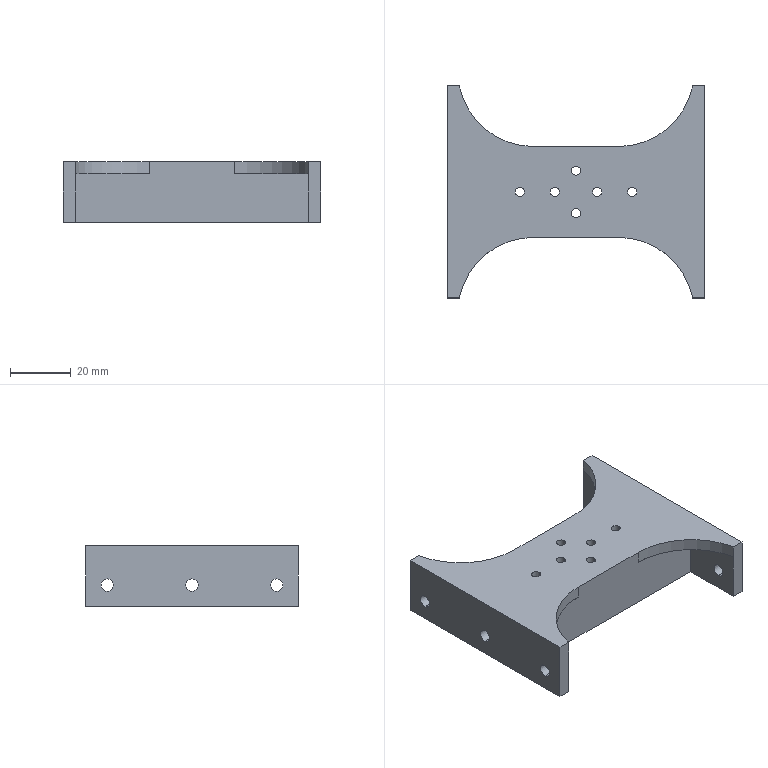Part | STEP file | Servo connection frame | 1 solid | 51 faces | box 85 x 70 x 20 mm | volume 29316 mm3 | cylinder 28 | plane 23 | commonest cylinder face diameters 3 x12 4.1 x12 50 x4